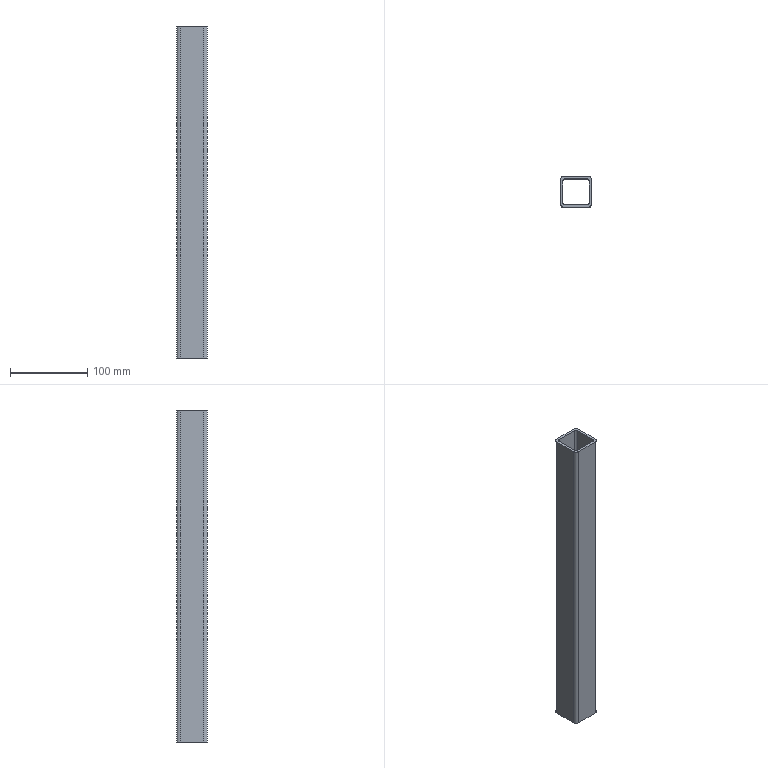Part | STEP file | DIN EN 10210-2 - 40 x 40 x 3 - 800 | 1 solid | 18 faces | box 40 x 40 x 429 mm | volume 186333 mm3 | plane 10 | cylinder 8 | commonest cylinder face diameters 6 x4 9 x4
STEP:
#1=CARTESIAN_POINT('',(0.,0.,0.));
#2=DIRECTION('',(0.,0.,1.));
#3=DIRECTION('',(1.,0.,0.));
#4=AXIS2_PLACEMENT_3D('',#1,#2,#3);
#5=CARTESIAN_POINT('',(17.,14.,0.));
#6=VERTEX_POINT('',#5);
#7=CARTESIAN_POINT('',(17.,14.,429.));
#8=VERTEX_POINT('',#7);
#9=CARTESIAN_POINT('',(17.,14.,0.));
#10=DIRECTION('',(0.,0.,1.));
#11=VECTOR('',#10,1.);
#12=LINE('',#9,#11);
#13=CARTESIAN_POINT('',(14.,14.,0.));
#14=DIRECTION('',(0.,0.,1.));
#15=DIRECTION('',(1.,0.,0.));
#16=AXIS2_PLACEMENT_3D('',#13,#14,#15);
#17=CYLINDRICAL_SURFACE('',#16,3.);
#18=CARTESIAN_POINT('',(0.,0.));
#19=DIRECTION('',(0.,1.));
#20=VECTOR('',#19,1.);
#21=LINE('',#18,#20);
#22=(GEOMETRIC_REPRESENTATION_CONTEXT(2)PARAMETRIC_REPRESENTATION_CONTEXT()REPRESENTATION_CONTEXT('',''));
#23=DEFINITIONAL_REPRESENTATION('',(#21),#22);
#24=PCURVE('',#17,#23);
#25=CARTESIAN_POINT('',(17.,14.,0.));
#26=DIRECTION('',(1.,0.,0.));
#27=DIRECTION('',(0.,0.,-1.));
#28=AXIS2_PLACEMENT_3D('',#25,#26,#27);
#29=PLANE('',#28);
#30=CARTESIAN_POINT('',(0.,0.));
#31=DIRECTION('',(-1.,0.));
#32=VECTOR('',#31,1.);
#33=LINE('',#30,#32);
#34=(GEOMETRIC_REPRESENTATION_CONTEXT(2)PARAMETRIC_REPRESENTATION_CONTEXT()REPRESENTATION_CONTEXT('',''));
#35=DEFINITIONAL_REPRESENTATION('',(#33),#34);
#36=PCURVE('',#29,#35);
#37=SURFACE_CURVE('',#12,(#24,#36),.PCURVE_S1.);
#38=EDGE_CURVE('',#6,#8,#37,.T.);
#39=ORIENTED_EDGE('',*,*,#38,.F.);
#40=CARTESIAN_POINT('',(14.,17.,0.));
#41=VERTEX_POINT('',#40);
#42=CARTESIAN_POINT('',(14.,14.,0.));
#43=DIRECTION('',(0.,0.,1.));
#44=DIRECTION('',(1.,0.,0.));
#45=AXIS2_PLACEMENT_3D('',#42,#43,#44);
#46=CIRCLE('',#45,3.);
#47=CARTESIAN_POINT('',(0.,0.));
#48=DIRECTION('',(1.,0.));
#49=VECTOR('',#48,1.);
#50=LINE('',#47,#49);
#51=(GEOMETRIC_REPRESENTATION_CONTEXT(2)PARAMETRIC_REPRESENTATION_CONTEXT()REPRESENTATION_CONTEXT('',''));
#52=DEFINITIONAL_REPRESENTATION('',(#50),#51);
#53=PCURVE('',#17,#52);
#54=CARTESIAN_POINT('',(0.,0.,0.));
#55=DIRECTION('',(0.,0.,1.));
#56=DIRECTION('',(1.,0.,0.));
#57=AXIS2_PLACEMENT_3D('',#54,#55,#56);
#58=PLANE('',#57);
#59=CARTESIAN_POINT('',(14.,14.));
#60=DIRECTION('',(1.,0.));
#61=AXIS2_PLACEMENT_2D('',#59,#60);
#62=CIRCLE('',#61,3.);
#63=(GEOMETRIC_REPRESENTATION_CONTEXT(2)PARAMETRIC_REPRESENTATION_CONTEXT()REPRESENTATION_CONTEXT('',''));
#64=DEFINITIONAL_REPRESENTATION('',(#62),#63);
#65=PCURVE('',#58,#64);
#66=SURFACE_CURVE('',#46,(#53,#65),.PCURVE_S1.);
#67=EDGE_CURVE('',#6,#41,#66,.T.);
#68=ORIENTED_EDGE('',*,*,#67,.T.);
#69=CARTESIAN_POINT('',(14.,17.,429.));
#70=VERTEX_POINT('',#69);
#71=CARTESIAN_POINT('',(14.,17.,0.));
#72=DIRECTION('',(0.,0.,1.));
#73=VECTOR('',#72,1.);
#74=LINE('',#71,#73);
#75=CARTESIAN_POINT('',(1.571,0.));
#76=DIRECTION('',(0.,1.));
#77=VECTOR('',#76,1.);
#78=LINE('',#75,#77);
#79=(GEOMETRIC_REPRESENTATION_CONTEXT(2)PARAMETRIC_REPRESENTATION_CONTEXT()REPRESENTATION_CONTEXT('',''));
#80=DEFINITIONAL_REPRESENTATION('',(#78),#79);
#81=PCURVE('',#17,#80);
#82=CARTESIAN_POINT('',(-14.,17.,0.));
#83=DIRECTION('',(0.,1.,0.));
#84=DIRECTION('',(0.,0.,1.));
#85=AXIS2_PLACEMENT_3D('',#82,#83,#84);
#86=PLANE('',#85);
#87=CARTESIAN_POINT('',(0.,28.));
#88=DIRECTION('',(1.,0.));
#89=VECTOR('',#88,1.);
#90=LINE('',#87,#89);
#91=(GEOMETRIC_REPRESENTATION_CONTEXT(2)PARAMETRIC_REPRESENTATION_CONTEXT()REPRESENTATION_CONTEXT('',''));
#92=DEFINITIONAL_REPRESENTATION('',(#90),#91);
#93=PCURVE('',#86,#92);
#94=SURFACE_CURVE('',#74,(#81,#93),.PCURVE_S1.);
#95=EDGE_CURVE('',#41,#70,#94,.T.);
#96=ORIENTED_EDGE('',*,*,#95,.T.);
#97=CARTESIAN_POINT('',(14.,14.,429.));
#98=DIRECTION('',(0.,0.,1.));
#99=DIRECTION('',(1.,0.,0.));
#100=AXIS2_PLACEMENT_3D('',#97,#98,#99);
#101=CIRCLE('',#100,3.);
#102=CARTESIAN_POINT('',(0.,429.));
#103=DIRECTION('',(1.,0.));
#104=VECTOR('',#103,1.);
#105=LINE('',#102,#104);
#106=(GEOMETRIC_REPRESENTATION_CONTEXT(2)PARAMETRIC_REPRESENTATION_CONTEXT()REPRESENTATION_CONTEXT('',''));
#107=DEFINITIONAL_REPRESENTATION('',(#105),#106);
#108=PCURVE('',#17,#107);
#109=CARTESIAN_POINT('',(0.,0.,429.));
#110=DIRECTION('',(0.,0.,1.));
#111=DIRECTION('',(1.,0.,0.));
#112=AXIS2_PLACEMENT_3D('',#109,#110,#111);
#113=PLANE('',#112);
#114=CARTESIAN_POINT('',(14.,14.));
#115=DIRECTION('',(1.,0.));
#116=AXIS2_PLACEMENT_2D('',#114,#115);
#117=CIRCLE('',#116,3.);
#118=(GEOMETRIC_REPRESENTATION_CONTEXT(2)PARAMETRIC_REPRESENTATION_CONTEXT()REPRESENTATION_CONTEXT('',''));
#119=DEFINITIONAL_REPRESENTATION('',(#117),#118);
#120=PCURVE('',#113,#119);
#121=SURFACE_CURVE('',#101,(#108,#120),.PCURVE_S1.);
#122=EDGE_CURVE('',#8,#70,#121,.T.);
#123=ORIENTED_EDGE('',*,*,#122,.F.);
#124=EDGE_LOOP('',(#39,#68,#96,#123));
#125=FACE_BOUND('',#124,.F.);
#126=ADVANCED_FACE('',(#125),#17,.F.);
#127=CARTESIAN_POINT('',(-14.,17.,429.));
#128=VERTEX_POINT('',#127);
#129=CARTESIAN_POINT('',(-7.,17.,429.));
#130=DIRECTION('',(-1.,0.,0.));
#131=VECTOR('',#130,1.);
#132=LINE('',#129,#131);
#133=CARTESIAN_POINT('',(429.,7.));
#134=DIRECTION('',(0.,-1.));
#135=VECTOR('',#134,1.);
#136=LINE('',#133,#135);
#137=(GEOMETRIC_REPRESENTATION_CONTEXT(2)PARAMETRIC_REPRESENTATION_CONTEXT()REPRESENTATION_CONTEXT('',''));
#138=DEFINITIONAL_REPRESENTATION('',(#136),#137);
#139=PCURVE('',#86,#138);
#140=CARTESIAN_POINT('',(-7.,17.));
#141=DIRECTION('',(-1.,0.));
#142=VECTOR('',#141,1.);
#143=LINE('',#140,#142);
#144=(GEOMETRIC_REPRESENTATION_CONTEXT(2)PARAMETRIC_REPRESENTATION_CONTEXT()REPRESENTATION_CONTEXT('',''));
#145=DEFINITIONAL_REPRESENTATION('',(#143),#144);
#146=PCURVE('',#113,#145);
#147=SURFACE_CURVE('',#132,(#139,#146),.PCURVE_S1.);
#148=EDGE_CURVE('',#70,#128,#147,.T.);
#149=ORIENTED_EDGE('',*,*,#148,.T.);
#150=CARTESIAN_POINT('',(-14.,17.,0.));
#151=VERTEX_POINT('',#150);
#152=CARTESIAN_POINT('',(-14.,17.,0.));
#153=DIRECTION('',(0.,0.,1.));
#154=VECTOR('',#153,1.);
#155=LINE('',#152,#154);
#156=CARTESIAN_POINT('',(0.,0.));
#157=DIRECTION('',(1.,0.));
#158=VECTOR('',#157,1.);
#159=LINE('',#156,#158);
#160=(GEOMETRIC_REPRESENTATION_CONTEXT(2)PARAMETRIC_REPRESENTATION_CONTEXT()REPRESENTATION_CONTEXT('',''));
#161=DEFINITIONAL_REPRESENTATION('',(#159),#160);
#162=PCURVE('',#86,#161);
#163=CARTESIAN_POINT('',(-14.,14.,0.));
#164=DIRECTION('',(0.,0.,1.));
#165=DIRECTION('',(0.,1.,0.));
#166=AXIS2_PLACEMENT_3D('',#163,#164,#165);
#167=CYLINDRICAL_SURFACE('',#166,3.);
#168=CARTESIAN_POINT('',(0.,0.));
#169=DIRECTION('',(0.,1.));
#170=VECTOR('',#169,1.);
#171=LINE('',#168,#170);
#172=(GEOMETRIC_REPRESENTATION_CONTEXT(2)PARAMETRIC_REPRESENTATION_CONTEXT()REPRESENTATION_CONTEXT('',''));
#173=DEFINITIONAL_REPRESENTATION('',(#171),#172);
#174=PCURVE('',#167,#173);
#175=SURFACE_CURVE('',#155,(#162,#174),.PCURVE_S1.);
#176=EDGE_CURVE('',#151,#128,#175,.T.);
#177=ORIENTED_EDGE('',*,*,#176,.F.);
#178=CARTESIAN_POINT('',(-7.,17.,0.));
#179=DIRECTION('',(-1.,0.,0.));
#180=VECTOR('',#179,1.);
#181=LINE('',#178,#180);
#182=CARTESIAN_POINT('',(0.,7.));
#183=DIRECTION('',(0.,-1.));
#184=VECTOR('',#183,1.);
#185=LINE('',#182,#184);
#186=(GEOMETRIC_REPRESENTATION_CONTEXT(2)PARAMETRIC_REPRESENTATION_CONTEXT()REPRESENTATION_CONTEXT('',''));
#187=DEFINITIONAL_REPRESENTATION('',(#185),#186);
#188=PCURVE('',#86,#187);
#189=CARTESIAN_POINT('',(-7.,17.));
#190=DIRECTION('',(-1.,0.));
#191=VECTOR('',#190,1.);
#192=LINE('',#189,#191);
#193=(GEOMETRIC_REPRESENTATION_CONTEXT(2)PARAMETRIC_REPRESENTATION_CONTEXT()REPRESENTATION_CONTEXT('',''));
#194=DEFINITIONAL_REPRESENTATION('',(#192),#193);
#195=PCURVE('',#58,#194);
#196=SURFACE_CURVE('',#181,(#188,#195),.PCURVE_S1.);
#197=EDGE_CURVE('',#41,#151,#196,.T.);
#198=ORIENTED_EDGE('',*,*,#197,.F.);
#199=ORIENTED_EDGE('',*,*,#95,.T.);
#200=EDGE_LOOP('',(#149,#177,#198,#199));
#201=FACE_BOUND('',#200,.T.);
#202=ADVANCED_FACE('',(#201),#86,.F.);
#203=ORIENTED_EDGE('',*,*,#176,.F.);
#204=CARTESIAN_POINT('',(-17.,14.,0.));
#205=VERTEX_POINT('',#204);
#206=CARTESIAN_POINT('',(-14.,14.,0.));
#207=DIRECTION('',(0.,0.,1.));
#208=DIRECTION('',(0.,1.,0.));
#209=AXIS2_PLACEMENT_3D('',#206,#207,#208);
#210=CIRCLE('',#209,3.);
#211=CARTESIAN_POINT('',(0.,0.));
#212=DIRECTION('',(1.,0.));
#213=VECTOR('',#212,1.);
#214=LINE('',#211,#213);
#215=(GEOMETRIC_REPRESENTATION_CONTEXT(2)PARAMETRIC_REPRESENTATION_CONTEXT()REPRESENTATION_CONTEXT('',''));
#216=DEFINITIONAL_REPRESENTATION('',(#214),#215);
#217=PCURVE('',#167,#216);
#218=CARTESIAN_POINT('',(-14.,14.));
#219=DIRECTION('',(0.,1.));
#220=AXIS2_PLACEMENT_2D('',#218,#219);
#221=CIRCLE('',#220,3.);
#222=(GEOMETRIC_REPRESENTATION_CONTEXT(2)PARAMETRIC_REPRESENTATION_CONTEXT()REPRESENTATION_CONTEXT('',''));
#223=DEFINITIONAL_REPRESENTATION('',(#221),#222);
#224=PCURVE('',#58,#223);
#225=SURFACE_CURVE('',#210,(#217,#224),.PCURVE_S1.);
#226=EDGE_CURVE('',#151,#205,#225,.T.);
#227=ORIENTED_EDGE('',*,*,#226,.T.);
#228=CARTESIAN_POINT('',(-17.,14.,429.));
#229=VERTEX_POINT('',#228);
#230=CARTESIAN_POINT('',(-17.,14.,0.));
#231=DIRECTION('',(0.,0.,1.));
#232=VECTOR('',#231,1.);
#233=LINE('',#230,#232);
#234=CARTESIAN_POINT('',(1.571,0.));
#235=DIRECTION('',(0.,1.));
#236=VECTOR('',#235,1.);
#237=LINE('',#234,#236);
#238=(GEOMETRIC_REPRESENTATION_CONTEXT(2)PARAMETRIC_REPRESENTATION_CONTEXT()REPRESENTATION_CONTEXT('',''));
#239=DEFINITIONAL_REPRESENTATION('',(#237),#238);
#240=PCURVE('',#167,#239);
#241=CARTESIAN_POINT('',(-17.,-14.,0.));
#242=DIRECTION('',(-1.,0.,0.));
#243=DIRECTION('',(0.,0.,1.));
#244=AXIS2_PLACEMENT_3D('',#241,#242,#243);
#245=PLANE('',#244);
#246=CARTESIAN_POINT('',(0.,28.));
#247=DIRECTION('',(1.,0.));
#248=VECTOR('',#247,1.);
#249=LINE('',#246,#248);
#250=(GEOMETRIC_REPRESENTATION_CONTEXT(2)PARAMETRIC_REPRESENTATION_CONTEXT()REPRESENTATION_CONTEXT('',''));
#251=DEFINITIONAL_REPRESENTATION('',(#249),#250);
#252=PCURVE('',#245,#251);
#253=SURFACE_CURVE('',#233,(#240,#252),.PCURVE_S1.);
#254=EDGE_CURVE('',#205,#229,#253,.T.);
#255=ORIENTED_EDGE('',*,*,#254,.T.);
#256=CARTESIAN_POINT('',(-14.,14.,429.));
#257=DIRECTION('',(0.,0.,1.));
#258=DIRECTION('',(0.,1.,0.));
#259=AXIS2_PLACEMENT_3D('',#256,#257,#258);
#260=CIRCLE('',#259,3.);
#261=CARTESIAN_POINT('',(0.,429.));
#262=DIRECTION('',(1.,0.));
#263=VECTOR('',#262,1.);
#264=LINE('',#261,#263);
#265=(GEOMETRIC_REPRESENTATION_CONTEXT(2)PARAMETRIC_REPRESENTATION_CONTEXT()REPRESENTATION_CONTEXT('',''));
#266=DEFINITIONAL_REPRESENTATION('',(#264),#265);
#267=PCURVE('',#167,#266);
#268=CARTESIAN_POINT('',(-14.,14.));
#269=DIRECTION('',(0.,1.));
#270=AXIS2_PLACEMENT_2D('',#268,#269);
#271=CIRCLE('',#270,3.);
#272=(GEOMETRIC_REPRESENTATION_CONTEXT(2)PARAMETRIC_REPRESENTATION_CONTEXT()REPRESENTATION_CONTEXT('',''));
#273=DEFINITIONAL_REPRESENTATION('',(#271),#272);
#274=PCURVE('',#113,#273);
#275=SURFACE_CURVE('',#260,(#267,#274),.PCURVE_S1.);
#276=EDGE_CURVE('',#128,#229,#275,.T.);
#277=ORIENTED_EDGE('',*,*,#276,.F.);
#278=EDGE_LOOP('',(#203,#227,#255,#277));
#279=FACE_BOUND('',#278,.F.);
#280=ADVANCED_FACE('',(#279),#167,.F.);
#281=CARTESIAN_POINT('',(-17.,-14.,429.));
#282=VERTEX_POINT('',#281);
#283=CARTESIAN_POINT('',(-17.,-7.,429.));
#284=DIRECTION('',(0.,-1.,0.));
#285=VECTOR('',#284,1.);
#286=LINE('',#283,#285);
#287=CARTESIAN_POINT('',(429.,7.));
#288=DIRECTION('',(0.,-1.));
#289=VECTOR('',#288,1.);
#290=LINE('',#287,#289);
#291=(GEOMETRIC_REPRESENTATION_CONTEXT(2)PARAMETRIC_REPRESENTATION_CONTEXT()REPRESENTATION_CONTEXT('',''));
#292=DEFINITIONAL_REPRESENTATION('',(#290),#291);
#293=PCURVE('',#245,#292);
#294=CARTESIAN_POINT('',(-17.,-7.));
#295=DIRECTION('',(0.,-1.));
#296=VECTOR('',#295,1.);
#297=LINE('',#294,#296);
#298=(GEOMETRIC_REPRESENTATION_CONTEXT(2)PARAMETRIC_REPRESENTATION_CONTEXT()REPRESENTATION_CONTEXT('',''));
#299=DEFINITIONAL_REPRESENTATION('',(#297),#298);
#300=PCURVE('',#113,#299);
#301=SURFACE_CURVE('',#286,(#293,#300),.PCURVE_S1.);
#302=EDGE_CURVE('',#229,#282,#301,.T.);
#303=ORIENTED_EDGE('',*,*,#302,.T.);
#304=CARTESIAN_POINT('',(-17.,-14.,0.));
#305=VERTEX_POINT('',#304);
#306=CARTESIAN_POINT('',(-17.,-14.,0.));
#307=DIRECTION('',(0.,0.,1.));
#308=VECTOR('',#307,1.);
#309=LINE('',#306,#308);
#310=CARTESIAN_POINT('',(0.,0.));
#311=DIRECTION('',(1.,0.));
#312=VECTOR('',#311,1.);
#313=LINE('',#310,#312);
#314=(GEOMETRIC_REPRESENTATION_CONTEXT(2)PARAMETRIC_REPRESENTATION_CONTEXT()REPRESENTATION_CONTEXT('',''));
#315=DEFINITIONAL_REPRESENTATION('',(#313),#314);
#316=PCURVE('',#245,#315);
#317=CARTESIAN_POINT('',(-14.,-14.,0.));
#318=DIRECTION('',(0.,0.,1.));
#319=DIRECTION('',(-1.,0.,0.));
#320=AXIS2_PLACEMENT_3D('',#317,#318,#319);
#321=CYLINDRICAL_SURFACE('',#320,3.);
#322=CARTESIAN_POINT('',(0.,0.));
#323=DIRECTION('',(0.,1.));
#324=VECTOR('',#323,1.);
#325=LINE('',#322,#324);
#326=(GEOMETRIC_REPRESENTATION_CONTEXT(2)PARAMETRIC_REPRESENTATION_CONTEXT()REPRESENTATION_CONTEXT('',''));
#327=DEFINITIONAL_REPRESENTATION('',(#325),#326);
#328=PCURVE('',#321,#327);
#329=SURFACE_CURVE('',#309,(#316,#328),.PCURVE_S1.);
#330=EDGE_CURVE('',#305,#282,#329,.T.);
#331=ORIENTED_EDGE('',*,*,#330,.F.);
#332=CARTESIAN_POINT('',(-17.,-7.,0.));
#333=DIRECTION('',(0.,-1.,0.));
#334=VECTOR('',#333,1.);
#335=LINE('',#332,#334);
#336=CARTESIAN_POINT('',(0.,7.));
#337=DIRECTION('',(0.,-1.));
#338=VECTOR('',#337,1.);
#339=LINE('',#336,#338);
#340=(GEOMETRIC_REPRESENTATION_CONTEXT(2)PARAMETRIC_REPRESENTATION_CONTEXT()REPRESENTATION_CONTEXT('',''));
#341=DEFINITIONAL_REPRESENTATION('',(#339),#340);
#342=PCURVE('',#245,#341);
#343=CARTESIAN_POINT('',(-17.,-7.));
#344=DIRECTION('',(0.,-1.));
#345=VECTOR('',#344,1.);
#346=LINE('',#343,#345);
#347=(GEOMETRIC_REPRESENTATION_CONTEXT(2)PARAMETRIC_REPRESENTATION_CONTEXT()REPRESENTATION_CONTEXT('',''));
#348=DEFINITIONAL_REPRESENTATION('',(#346),#347);
#349=PCURVE('',#58,#348);
#350=SURFACE_CURVE('',#335,(#342,#349),.PCURVE_S1.);
#351=EDGE_CURVE('',#205,#305,#350,.T.);
#352=ORIENTED_EDGE('',*,*,#351,.F.);
#353=ORIENTED_EDGE('',*,*,#254,.T.);
#354=EDGE_LOOP('',(#303,#331,#352,#353));
#355=FACE_BOUND('',#354,.T.);
#356=ADVANCED_FACE('',(#355),#245,.F.);
#357=CARTESIAN_POINT('',(20.,15.5,429.));
#358=VERTEX_POINT('',#357);
#359=CARTESIAN_POINT('',(20.,-15.5,429.));
#360=VERTEX_POINT('',#359);
#361=CARTESIAN_POINT('',(20.,7.75,429.));
#362=DIRECTION('',(0.,-1.,0.));
#363=VECTOR('',#362,1.);
#364=LINE('',#361,#363);
#365=CARTESIAN_POINT('',(20.,15.5,0.));
#366=DIRECTION('',(1.,0.,0.));
#367=DIRECTION('',(0.,0.,-1.));
#368=AXIS2_PLACEMENT_3D('',#365,#366,#367);
#369=PLANE('',#368);
#370=CARTESIAN_POINT('',(-429.,-7.75));
#371=DIRECTION('',(0.,-1.));
#372=VECTOR('',#371,1.);
#373=LINE('',#370,#372);
#374=(GEOMETRIC_REPRESENTATION_CONTEXT(2)PARAMETRIC_REPRESENTATION_CONTEXT()REPRESENTATION_CONTEXT('',''));
#375=DEFINITIONAL_REPRESENTATION('',(#373),#374);
#376=PCURVE('',#369,#375);
#377=CARTESIAN_POINT('',(20.,7.75));
#378=DIRECTION('',(0.,-1.));
#379=VECTOR('',#378,1.);
#380=LINE('',#377,#379);
#381=(GEOMETRIC_REPRESENTATION_CONTEXT(2)PARAMETRIC_REPRESENTATION_CONTEXT()REPRESENTATION_CONTEXT('',''));
#382=DEFINITIONAL_REPRESENTATION('',(#380),#381);
#383=PCURVE('',#113,#382);
#384=SURFACE_CURVE('',#364,(#376,#383),.PCURVE_S1.);
#385=EDGE_CURVE('',#358,#360,#384,.T.);
#386=ORIENTED_EDGE('',*,*,#385,.T.);
#387=CARTESIAN_POINT('',(20.,-15.5,0.));
#388=VERTEX_POINT('',#387);
#389=CARTESIAN_POINT('',(20.,-15.5,0.));
#390=DIRECTION('',(0.,0.,1.));
#391=VECTOR('',#390,1.);
#392=LINE('',#389,#391);
#393=CARTESIAN_POINT('',(0.,-31.));
#394=DIRECTION('',(-1.,0.));
#395=VECTOR('',#394,1.);
#396=LINE('',#393,#395);
#397=(GEOMETRIC_REPRESENTATION_CONTEXT(2)PARAMETRIC_REPRESENTATION_CONTEXT()REPRESENTATION_CONTEXT('',''));
#398=DEFINITIONAL_REPRESENTATION('',(#396),#397);
#399=PCURVE('',#369,#398);
#400=CARTESIAN_POINT('',(15.5,-15.5,0.));
#401=DIRECTION('',(0.,0.,1.));
#402=DIRECTION('',(0.,1.,0.));
#403=AXIS2_PLACEMENT_3D('',#400,#401,#402);
#404=CYLINDRICAL_SURFACE('',#403,4.5);
#405=CARTESIAN_POINT('',(4.712,0.));
#406=DIRECTION('',(0.,1.));
#407=VECTOR('',#406,1.);
#408=LINE('',#405,#407);
#409=(GEOMETRIC_REPRESENTATION_CONTEXT(2)PARAMETRIC_REPRESENTATION_CONTEXT()REPRESENTATION_CONTEXT('',''));
#410=DEFINITIONAL_REPRESENTATION('',(#408),#409);
#411=PCURVE('',#404,#410);
#412=SURFACE_CURVE('',#392,(#399,#411),.PCURVE_S1.);
#413=EDGE_CURVE('',#388,#360,#412,.T.);
#414=ORIENTED_EDGE('',*,*,#413,.F.);
#415=CARTESIAN_POINT('',(20.,15.5,0.));
#416=VERTEX_POINT('',#415);
#417=CARTESIAN_POINT('',(20.,7.75,0.));
#418=DIRECTION('',(0.,-1.,0.));
#419=VECTOR('',#418,1.);
#420=LINE('',#417,#419);
#421=CARTESIAN_POINT('',(0.,-7.75));
#422=DIRECTION('',(0.,-1.));
#423=VECTOR('',#422,1.);
#424=LINE('',#421,#423);
#425=(GEOMETRIC_REPRESENTATION_CONTEXT(2)PARAMETRIC_REPRESENTATION_CONTEXT()REPRESENTATION_CONTEXT('',''));
#426=DEFINITIONAL_REPRESENTATION('',(#424),#425);
#427=PCURVE('',#369,#426);
#428=CARTESIAN_POINT('',(20.,7.75));
#429=DIRECTION('',(0.,-1.));
#430=VECTOR('',#429,1.);
#431=LINE('',#428,#430);
#432=(GEOMETRIC_REPRESENTATION_CONTEXT(2)PARAMETRIC_REPRESENTATION_CONTEXT()REPRESENTATION_CONTEXT('',''));
#433=DEFINITIONAL_REPRESENTATION('',(#431),#432);
#434=PCURVE('',#58,#433);
#435=SURFACE_CURVE('',#420,(#427,#434),.PCURVE_S1.);
#436=EDGE_CURVE('',#416,#388,#435,.T.);
#437=ORIENTED_EDGE('',*,*,#436,.F.);
#438=CARTESIAN_POINT('',(20.,15.5,0.));
#439=DIRECTION('',(0.,0.,1.));
#440=VECTOR('',#439,1.);
#441=LINE('',#438,#440);
#442=CARTESIAN_POINT('',(0.,0.));
#443=DIRECTION('',(-1.,0.));
#444=VECTOR('',#443,1.);
#445=LINE('',#442,#444);
#446=(GEOMETRIC_REPRESENTATION_CONTEXT(2)PARAMETRIC_REPRESENTATION_CONTEXT()REPRESENTATION_CONTEXT('',''));
#447=DEFINITIONAL_REPRESENTATION('',(#445),#446);
#448=PCURVE('',#369,#447);
#449=CARTESIAN_POINT('',(15.5,15.5,0.));
#450=DIRECTION('',(0.,0.,1.));
#451=DIRECTION('',(-1.,0.,0.));
#452=AXIS2_PLACEMENT_3D('',#449,#450,#451);
#453=CYLINDRICAL_SURFACE('',#452,4.5);
#454=CARTESIAN_POINT('',(3.142,0.));
#455=DIRECTION('',(0.,1.));
#456=VECTOR('',#455,1.);
#457=LINE('',#454,#456);
#458=(GEOMETRIC_REPRESENTATION_CONTEXT(2)PARAMETRIC_REPRESENTATION_CONTEXT()REPRESENTATION_CONTEXT('',''));
#459=DEFINITIONAL_REPRESENTATION('',(#457),#458);
#460=PCURVE('',#453,#459);
#461=SURFACE_CURVE('',#441,(#448,#460),.PCURVE_S1.);
#462=EDGE_CURVE('',#416,#358,#461,.T.);
#463=ORIENTED_EDGE('',*,*,#462,.T.);
#464=EDGE_LOOP('',(#386,#414,#437,#463));
#465=FACE_BOUND('',#464,.T.);
#466=ADVANCED_FACE('',(#465),#369,.T.);
#467=CARTESIAN_POINT('',(15.5,-20.,429.));
#468=VERTEX_POINT('',#467);
#469=CARTESIAN_POINT('',(15.5,-15.5,429.));
#470=DIRECTION('',(0.,0.,-1.));
#471=DIRECTION('',(0.,1.,0.));
#472=AXIS2_PLACEMENT_3D('',#469,#470,#471);
#473=CIRCLE('',#472,4.5);
#474=CARTESIAN_POINT('',(6.283,429.));
#475=DIRECTION('',(-1.,0.));
#476=VECTOR('',#475,1.);
#477=LINE('',#474,#476);
#478=(GEOMETRIC_REPRESENTATION_CONTEXT(2)PARAMETRIC_REPRESENTATION_CONTEXT()REPRESENTATION_CONTEXT('',''));
#479=DEFINITIONAL_REPRESENTATION('',(#477),#478);
#480=PCURVE('',#404,#479);
#481=CARTESIAN_POINT('',(15.5,-11.));
#482=CARTESIAN_POINT('',(23.294,-11.));
#483=CARTESIAN_POINT('',(19.397,-17.75));
#484=CARTESIAN_POINT('',(15.5,-24.5));
#485=CARTESIAN_POINT('',(11.603,-17.75));
#486=CARTESIAN_POINT('',(7.706,-11.));
#487=CARTESIAN_POINT('',(15.5,-11.));
#488=(BOUNDED_CURVE()B_SPLINE_CURVE(2,(#481,#482,#483,#484,#485,#486,#487),.UNSPECIFIED.,.T.,.F.)B_SPLINE_CURVE_WITH_KNOTS((1,2,2,2,2,1),(-2.094,0.,2.094,4.189,6.283,8.378),.UNSPECIFIED.)CURVE()GEOMETRIC_REPRESENTATION_ITEM()RATIONAL_B_SPLINE_CURVE((1.,0.5,1.,0.5,1.,0.5,1.))REPRESENTATION_ITEM(''));
#489=(GEOMETRIC_REPRESENTATION_CONTEXT(2)PARAMETRIC_REPRESENTATION_CONTEXT()REPRESENTATION_CONTEXT('',''));
#490=DEFINITIONAL_REPRESENTATION('',(#488),#489);
#491=PCURVE('',#113,#490);
#492=SURFACE_CURVE('',#473,(#480,#491),.PCURVE_S1.);
#493=EDGE_CURVE('',#360,#468,#492,.T.);
#494=ORIENTED_EDGE('',*,*,#493,.T.);
#495=CARTESIAN_POINT('',(15.5,-20.,0.));
#496=VERTEX_POINT('',#495);
#497=CARTESIAN_POINT('',(15.5,-20.,0.));
#498=DIRECTION('',(0.,0.,1.));
#499=VECTOR('',#498,1.);
#500=LINE('',#497,#499);
#501=CARTESIAN_POINT('',(3.142,0.));
#502=DIRECTION('',(0.,1.));
#503=VECTOR('',#502,1.);
#504=LINE('',#501,#503);
#505=(GEOMETRIC_REPRESENTATION_CONTEXT(2)PARAMETRIC_REPRESENTATION_CONTEXT()REPRESENTATION_CONTEXT('',''));
#506=DEFINITIONAL_REPRESENTATION('',(#504),#505);
#507=PCURVE('',#404,#506);
#508=CARTESIAN_POINT('',(15.5,-20.,0.));
#509=DIRECTION('',(0.,-1.,0.));
#510=DIRECTION('',(0.,0.,-1.));
#511=AXIS2_PLACEMENT_3D('',#508,#509,#510);
#512=PLANE('',#511);
#513=CARTESIAN_POINT('',(0.,0.));
#514=DIRECTION('',(-1.,0.));
#515=VECTOR('',#514,1.);
#516=LINE('',#513,#515);
#517=(GEOMETRIC_REPRESENTATION_CONTEXT(2)PARAMETRIC_REPRESENTATION_CONTEXT()REPRESENTATION_CONTEXT('',''));
#518=DEFINITIONAL_REPRESENTATION('',(#516),#517);
#519=PCURVE('',#512,#518);
#520=SURFACE_CURVE('',#500,(#507,#519),.PCURVE_S1.);
#521=EDGE_CURVE('',#496,#468,#520,.T.);
#522=ORIENTED_EDGE('',*,*,#521,.F.);
#523=CARTESIAN_POINT('',(15.5,-15.5,0.));
#524=DIRECTION('',(0.,0.,-1.));
#525=DIRECTION('',(0.,1.,0.));
#526=AXIS2_PLACEMENT_3D('',#523,#524,#525);
#527=CIRCLE('',#526,4.5);
#528=CARTESIAN_POINT('',(6.283,0.));
#529=DIRECTION('',(-1.,0.));
#530=VECTOR('',#529,1.);
#531=LINE('',#528,#530);
#532=(GEOMETRIC_REPRESENTATION_CONTEXT(2)PARAMETRIC_REPRESENTATION_CONTEXT()REPRESENTATION_CONTEXT('',''));
#533=DEFINITIONAL_REPRESENTATION('',(#531),#532);
#534=PCURVE('',#404,#533);
#535=CARTESIAN_POINT('',(15.5,-11.));
#536=CARTESIAN_POINT('',(23.294,-11.));
#537=CARTESIAN_POINT('',(19.397,-17.75));
#538=CARTESIAN_POINT('',(15.5,-24.5));
#539=CARTESIAN_POINT('',(11.603,-17.75));
#540=CARTESIAN_POINT('',(7.706,-11.));
#541=CARTESIAN_POINT('',(15.5,-11.));
#542=(BOUNDED_CURVE()B_SPLINE_CURVE(2,(#535,#536,#537,#538,#539,#540,#541),.UNSPECIFIED.,.T.,.F.)B_SPLINE_CURVE_WITH_KNOTS((1,2,2,2,2,1),(-2.094,0.,2.094,4.189,6.283,8.378),.UNSPECIFIED.)CURVE()GEOMETRIC_REPRESENTATION_ITEM()RATIONAL_B_SPLINE_CURVE((1.,0.5,1.,0.5,1.,0.5,1.))REPRESENTATION_ITEM(''));
#543=(GEOMETRIC_REPRESENTATION_CONTEXT(2)PARAMETRIC_REPRESENTATION_CONTEXT()REPRESENTATION_CONTEXT('',''));
#544=DEFINITIONAL_REPRESENTATION('',(#542),#543);
#545=PCURVE('',#58,#544);
#546=SURFACE_CURVE('',#527,(#534,#545),.PCURVE_S1.);
#547=EDGE_CURVE('',#388,#496,#546,.T.);
#548=ORIENTED_EDGE('',*,*,#547,.F.);
#549=ORIENTED_EDGE('',*,*,#413,.T.);
#550=EDGE_LOOP('',(#494,#522,#548,#549));
#551=FACE_BOUND('',#550,.T.);
#552=ADVANCED_FACE('',(#551),#404,.T.);
#553=CARTESIAN_POINT('',(-15.5,-20.,429.));
#554=VERTEX_POINT('',#553);
#555=CARTESIAN_POINT('',(7.75,-20.,429.));
#556=DIRECTION('',(-1.,0.,0.));
#557=VECTOR('',#556,1.);
#558=LINE('',#555,#557);
#559=CARTESIAN_POINT('',(-429.,-7.75));
#560=DIRECTION('',(0.,-1.));
#561=VECTOR('',#560,1.);
#562=LINE('',#559,#561);
#563=(GEOMETRIC_REPRESENTATION_CONTEXT(2)PARAMETRIC_REPRESENTATION_CONTEXT()REPRESENTATION_CONTEXT('',''));
#564=DEFINITIONAL_REPRESENTATION('',(#562),#563);
#565=PCURVE('',#512,#564);
#566=CARTESIAN_POINT('',(7.75,-20.));
#567=DIRECTION('',(-1.,0.));
#568=VECTOR('',#567,1.);
#569=LINE('',#566,#568);
#570=(GEOMETRIC_REPRESENTATION_CONTEXT(2)PARAMETRIC_REPRESENTATION_CONTEXT()REPRESENTATION_CONTEXT('',''));
#571=DEFINITIONAL_REPRESENTATION('',(#569),#570);
#572=PCURVE('',#113,#571);
#573=SURFACE_CURVE('',#558,(#565,#572),.PCURVE_S1.);
#574=EDGE_CURVE('',#468,#554,#573,.T.);
#575=ORIENTED_EDGE('',*,*,#574,.T.);
#576=CARTESIAN_POINT('',(-15.5,-20.,0.));
#577=VERTEX_POINT('',#576);
#578=CARTESIAN_POINT('',(-15.5,-20.,0.));
#579=DIRECTION('',(0.,0.,1.));
#580=VECTOR('',#579,1.);
#581=LINE('',#578,#580);
#582=CARTESIAN_POINT('',(0.,-31.));
#583=DIRECTION('',(-1.,0.));
#584=VECTOR('',#583,1.);
#585=LINE('',#582,#584);
#586=(GEOMETRIC_REPRESENTATION_CONTEXT(2)PARAMETRIC_REPRESENTATION_CONTEXT()REPRESENTATION_CONTEXT('',''));
#587=DEFINITIONAL_REPRESENTATION('',(#585),#586);
#588=PCURVE('',#512,#587);
#589=CARTESIAN_POINT('',(-15.5,-15.5,0.));
#590=DIRECTION('',(0.,0.,1.));
#591=DIRECTION('',(1.,0.,0.));
#592=AXIS2_PLACEMENT_3D('',#589,#590,#591);
#593=CYLINDRICAL_SURFACE('',#592,4.5);
#594=CARTESIAN_POINT('',(4.712,0.));
#595=DIRECTION('',(0.,1.));
#596=VECTOR('',#595,1.);
#597=LINE('',#594,#596);
#598=(GEOMETRIC_REPRESENTATION_CONTEXT(2)PARAMETRIC_REPRESENTATION_CONTEXT()REPRESENTATION_CONTEXT('',''));
#599=DEFINITIONAL_REPRESENTATION('',(#597),#598);
#600=PCURVE('',#593,#599);
#601=SURFACE_CURVE('',#581,(#588,#600),.PCURVE_S1.);
#602=EDGE_CURVE('',#577,#554,#601,.T.);
#603=ORIENTED_EDGE('',*,*,#602,.F.);
#604=CARTESIAN_POINT('',(7.75,-20.,0.));
#605=DIRECTION('',(-1.,0.,0.));
#606=VECTOR('',#605,1.);
#607=LINE('',#604,#606);
#608=CARTESIAN_POINT('',(0.,-7.75));
#609=DIRECTION('',(0.,-1.));
#610=VECTOR('',#609,1.);
#611=LINE('',#608,#610);
#612=(GEOMETRIC_REPRESENTATION_CONTEXT(2)PARAMETRIC_REPRESENTATION_CONTEXT()REPRESENTATION_CONTEXT('',''));
#613=DEFINITIONAL_REPRESENTATION('',(#611),#612);
#614=PCURVE('',#512,#613);
#615=CARTESIAN_POINT('',(7.75,-20.));
#616=DIRECTION('',(-1.,0.));
#617=VECTOR('',#616,1.);
#618=LINE('',#615,#617);
#619=(GEOMETRIC_REPRESENTATION_CONTEXT(2)PARAMETRIC_REPRESENTATION_CONTEXT()REPRESENTATION_CONTEXT('',''));
#620=DEFINITIONAL_REPRESENTATION('',(#618),#619);
#621=PCURVE('',#58,#620);
#622=SURFACE_CURVE('',#607,(#614,#621),.PCURVE_S1.);
#623=EDGE_CURVE('',#496,#577,#622,.T.);
#624=ORIENTED_EDGE('',*,*,#623,.F.);
#625=ORIENTED_EDGE('',*,*,#521,.T.);
#626=EDGE_LOOP('',(#575,#603,#624,#625));
#627=FACE_BOUND('',#626,.T.);
#628=ADVANCED_FACE('',(#627),#512,.T.);
#629=CARTESIAN_POINT('',(-20.,-15.5,429.));
#630=VERTEX_POINT('',#629);
#631=CARTESIAN_POINT('',(-15.5,-15.5,429.));
#632=DIRECTION('',(0.,0.,-1.));
#633=DIRECTION('',(1.,0.,0.));
#634=AXIS2_PLACEMENT_3D('',#631,#632,#633);
#635=CIRCLE('',#634,4.5);
#636=CARTESIAN_POINT('',(6.283,429.));
#637=DIRECTION('',(-1.,0.));
#638=VECTOR('',#637,1.);
#639=LINE('',#636,#638);
#640=(GEOMETRIC_REPRESENTATION_CONTEXT(2)PARAMETRIC_REPRESENTATION_CONTEXT()REPRESENTATION_CONTEXT('',''));
#641=DEFINITIONAL_REPRESENTATION('',(#639),#640);
#642=PCURVE('',#593,#641);
#643=CARTESIAN_POINT('',(-11.,-15.5));
#644=CARTESIAN_POINT('',(-11.,-23.294));
#645=CARTESIAN_POINT('',(-17.75,-19.397));
#646=CARTESIAN_POINT('',(-24.5,-15.5));
#647=CARTESIAN_POINT('',(-17.75,-11.603));
#648=CARTESIAN_POINT('',(-11.,-7.706));
#649=CARTESIAN_POINT('',(-11.,-15.5));
#650=(BOUNDED_CURVE()B_SPLINE_CURVE(2,(#643,#644,#645,#646,#647,#648,#649),.UNSPECIFIED.,.T.,.F.)B_SPLINE_CURVE_WITH_KNOTS((1,2,2,2,2,1),(-2.094,0.,2.094,4.189,6.283,8.378),.UNSPECIFIED.)CURVE()GEOMETRIC_REPRESENTATION_ITEM()RATIONAL_B_SPLINE_CURVE((1.,0.5,1.,0.5,1.,0.5,1.))REPRESENTATION_ITEM(''));
#651=(GEOMETRIC_REPRESENTATION_CONTEXT(2)PARAMETRIC_REPRESENTATION_CONTEXT()REPRESENTATION_CONTEXT('',''));
#652=DEFINITIONAL_REPRESENTATION('',(#650),#651);
#653=PCURVE('',#113,#652);
#654=SURFACE_CURVE('',#635,(#642,#653),.PCURVE_S1.);
#655=EDGE_CURVE('',#554,#630,#654,.T.);
#656=ORIENTED_EDGE('',*,*,#655,.T.);
#657=CARTESIAN_POINT('',(-20.,-15.5,0.));
#658=VERTEX_POINT('',#657);
#659=CARTESIAN_POINT('',(-20.,-15.5,0.));
#660=DIRECTION('',(0.,0.,1.));
#661=VECTOR('',#660,1.);
#662=LINE('',#659,#661);
#663=CARTESIAN_POINT('',(3.142,0.));
#664=DIRECTION('',(0.,1.));
#665=VECTOR('',#664,1.);
#666=LINE('',#663,#665);
#667=(GEOMETRIC_REPRESENTATION_CONTEXT(2)PARAMETRIC_REPRESENTATION_CONTEXT()REPRESENTATION_CONTEXT('',''));
#668=DEFINITIONAL_REPRESENTATION('',(#666),#667);
#669=PCURVE('',#593,#668);
#670=CARTESIAN_POINT('',(-20.,-15.5,0.));
#671=DIRECTION('',(-1.,0.,0.));
#672=DIRECTION('',(0.,0.,1.));
#673=AXIS2_PLACEMENT_3D('',#670,#671,#672);
#674=PLANE('',#673);
#675=CARTESIAN_POINT('',(0.,0.));
#676=DIRECTION('',(1.,0.));
#677=VECTOR('',#676,1.);
#678=LINE('',#675,#677);
#679=(GEOMETRIC_REPRESENTATION_CONTEXT(2)PARAMETRIC_REPRESENTATION_CONTEXT()REPRESENTATION_CONTEXT('',''));
#680=DEFINITIONAL_REPRESENTATION('',(#678),#679);
#681=PCURVE('',#674,#680);
#682=SURFACE_CURVE('',#662,(#669,#681),.PCURVE_S1.);
#683=EDGE_CURVE('',#658,#630,#682,.T.);
#684=ORIENTED_EDGE('',*,*,#683,.F.);
#685=CARTESIAN_POINT('',(-15.5,-15.5,0.));
#686=DIRECTION('',(0.,0.,-1.));
#687=DIRECTION('',(1.,0.,0.));
#688=AXIS2_PLACEMENT_3D('',#685,#686,#687);
#689=CIRCLE('',#688,4.5);
#690=CARTESIAN_POINT('',(6.283,0.));
#691=DIRECTION('',(-1.,0.));
#692=VECTOR('',#691,1.);
#693=LINE('',#690,#692);
#694=(GEOMETRIC_REPRESENTATION_CONTEXT(2)PARAMETRIC_REPRESENTATION_CONTEXT()REPRESENTATION_CONTEXT('',''));
#695=DEFINITIONAL_REPRESENTATION('',(#693),#694);
#696=PCURVE('',#593,#695);
#697=CARTESIAN_POINT('',(-11.,-15.5));
#698=CARTESIAN_POINT('',(-11.,-23.294));
#699=CARTESIAN_POINT('',(-17.75,-19.397));
#700=CARTESIAN_POINT('',(-24.5,-15.5));
#701=CARTESIAN_POINT('',(-17.75,-11.603));
#702=CARTESIAN_POINT('',(-11.,-7.706));
#703=CARTESIAN_POINT('',(-11.,-15.5));
#704=(BOUNDED_CURVE()B_SPLINE_CURVE(2,(#697,#698,#699,#700,#701,#702,#703),.UNSPECIFIED.,.T.,.F.)B_SPLINE_CURVE_WITH_KNOTS((1,2,2,2,2,1),(-2.094,0.,2.094,4.189,6.283,8.378),.UNSPECIFIED.)CURVE()GEOMETRIC_REPRESENTATION_ITEM()RATIONAL_B_SPLINE_CURVE((1.,0.5,1.,0.5,1.,0.5,1.))REPRESENTATION_ITEM(''));
#705=(GEOMETRIC_REPRESENTATION_CONTEXT(2)PARAMETRIC_REPRESENTATION_CONTEXT()REPRESENTATION_CONTEXT('',''));
#706=DEFINITIONAL_REPRESENTATION('',(#704),#705);
#707=PCURVE('',#58,#706);
#708=SURFACE_CURVE('',#689,(#696,#707),.PCURVE_S1.);
#709=EDGE_CURVE('',#577,#658,#708,.T.);
#710=ORIENTED_EDGE('',*,*,#709,.F.);
#711=ORIENTED_EDGE('',*,*,#602,.T.);
#712=EDGE_LOOP('',(#656,#684,#710,#711));
#713=FACE_BOUND('',#712,.T.);
#714=ADVANCED_FACE('',(#713),#593,.T.);
#715=ORIENTED_EDGE('',*,*,#330,.F.);
#716=CARTESIAN_POINT('',(-14.,-17.,0.));
#717=VERTEX_POINT('',#716);
#718=CARTESIAN_POINT('',(-14.,-14.,0.));
#719=DIRECTION('',(0.,0.,1.));
#720=DIRECTION('',(-1.,0.,0.));
#721=AXIS2_PLACEMENT_3D('',#718,#719,#720);
#722=CIRCLE('',#721,3.);
#723=CARTESIAN_POINT('',(0.,0.));
#724=DIRECTION('',(1.,0.));
#725=VECTOR('',#724,1.);
#726=LINE('',#723,#725);
#727=(GEOMETRIC_REPRESENTATION_CONTEXT(2)PARAMETRIC_REPRESENTATION_CONTEXT()REPRESENTATION_CONTEXT('',''));
#728=DEFINITIONAL_REPRESENTATION('',(#726),#727);
#729=PCURVE('',#321,#728);
#730=CARTESIAN_POINT('',(-14.,-14.));
#731=DIRECTION('',(-1.,0.));
#732=AXIS2_PLACEMENT_2D('',#730,#731);
#733=CIRCLE('',#732,3.);
#734=(GEOMETRIC_REPRESENTATION_CONTEXT(2)PARAMETRIC_REPRESENTATION_CONTEXT()REPRESENTATION_CONTEXT('',''));
#735=DEFINITIONAL_REPRESENTATION('',(#733),#734);
#736=PCURVE('',#58,#735);
#737=SURFACE_CURVE('',#722,(#729,#736),.PCURVE_S1.);
#738=EDGE_CURVE('',#305,#717,#737,.T.);
#739=ORIENTED_EDGE('',*,*,#738,.T.);
#740=CARTESIAN_POINT('',(-14.,-17.,429.));
#741=VERTEX_POINT('',#740);
#742=CARTESIAN_POINT('',(-14.,-17.,0.));
#743=DIRECTION('',(0.,0.,1.));
#744=VECTOR('',#743,1.);
#745=LINE('',#742,#744);
#746=CARTESIAN_POINT('',(1.571,0.));
#747=DIRECTION('',(0.,1.));
#748=VECTOR('',#747,1.);
#749=LINE('',#746,#748);
#750=(GEOMETRIC_REPRESENTATION_CONTEXT(2)PARAMETRIC_REPRESENTATION_CONTEXT()REPRESENTATION_CONTEXT('',''));
#751=DEFINITIONAL_REPRESENTATION('',(#749),#750);
#752=PCURVE('',#321,#751);
#753=CARTESIAN_POINT('',(14.,-17.,0.));
#754=DIRECTION('',(0.,-1.,0.));
#755=DIRECTION('',(0.,0.,-1.));
#756=AXIS2_PLACEMENT_3D('',#753,#754,#755);
#757=PLANE('',#756);
#758=CARTESIAN_POINT('',(0.,-28.));
#759=DIRECTION('',(-1.,0.));
#760=VECTOR('',#759,1.);
#761=LINE('',#758,#760);
#762=(GEOMETRIC_REPRESENTATION_CONTEXT(2)PARAMETRIC_REPRESENTATION_CONTEXT()REPRESENTATION_CONTEXT('',''));
#763=DEFINITIONAL_REPRESENTATION('',(#761),#762);
#764=PCURVE('',#757,#763);
#765=SURFACE_CURVE('',#745,(#752,#764),.PCURVE_S1.);
#766=EDGE_CURVE('',#717,#741,#765,.T.);
#767=ORIENTED_EDGE('',*,*,#766,.T.);
#768=CARTESIAN_POINT('',(-14.,-14.,429.));
#769=DIRECTION('',(0.,0.,1.));
#770=DIRECTION('',(-1.,0.,0.));
#771=AXIS2_PLACEMENT_3D('',#768,#769,#770);
#772=CIRCLE('',#771,3.);
#773=CARTESIAN_POINT('',(0.,429.));
#774=DIRECTION('',(1.,0.));
#775=VECTOR('',#774,1.);
#776=LINE('',#773,#775);
#777=(GEOMETRIC_REPRESENTATION_CONTEXT(2)PARAMETRIC_REPRESENTATION_CONTEXT()REPRESENTATION_CONTEXT('',''));
#778=DEFINITIONAL_REPRESENTATION('',(#776),#777);
#779=PCURVE('',#321,#778);
#780=CARTESIAN_POINT('',(-14.,-14.));
#781=DIRECTION('',(-1.,0.));
#782=AXIS2_PLACEMENT_2D('',#780,#781);
#783=CIRCLE('',#782,3.);
#784=(GEOMETRIC_REPRESENTATION_CONTEXT(2)PARAMETRIC_REPRESENTATION_CONTEXT()REPRESENTATION_CONTEXT('',''));
#785=DEFINITIONAL_REPRESENTATION('',(#783),#784);
#786=PCURVE('',#113,#785);
#787=SURFACE_CURVE('',#772,(#779,#786),.PCURVE_S1.);
#788=EDGE_CURVE('',#282,#741,#787,.T.);
#789=ORIENTED_EDGE('',*,*,#788,.F.);
#790=EDGE_LOOP('',(#715,#739,#767,#789));
#791=FACE_BOUND('',#790,.F.);
#792=ADVANCED_FACE('',(#791),#321,.F.);
#793=CARTESIAN_POINT('',(17.,-14.,429.));
#794=VERTEX_POINT('',#793);
#795=CARTESIAN_POINT('',(17.,7.,429.));
#796=DIRECTION('',(0.,1.,0.));
#797=VECTOR('',#796,1.);
#798=LINE('',#795,#797);
#799=CARTESIAN_POINT('',(-429.,-7.));
#800=DIRECTION('',(0.,1.));
#801=VECTOR('',#800,1.);
#802=LINE('',#799,#801);
#803=(GEOMETRIC_REPRESENTATION_CONTEXT(2)PARAMETRIC_REPRESENTATION_CONTEXT()REPRESENTATION_CONTEXT('',''));
#804=DEFINITIONAL_REPRESENTATION('',(#802),#803);
#805=PCURVE('',#29,#804);
#806=CARTESIAN_POINT('',(17.,7.));
#807=DIRECTION('',(0.,1.));
#808=VECTOR('',#807,1.);
#809=LINE('',#806,#808);
#810=(GEOMETRIC_REPRESENTATION_CONTEXT(2)PARAMETRIC_REPRESENTATION_CONTEXT()REPRESENTATION_CONTEXT('',''));
#811=DEFINITIONAL_REPRESENTATION('',(#809),#810);
#812=PCURVE('',#113,#811);
#813=SURFACE_CURVE('',#798,(#805,#812),.PCURVE_S1.);
#814=EDGE_CURVE('',#794,#8,#813,.T.);
#815=ORIENTED_EDGE('',*,*,#814,.T.);
#816=ORIENTED_EDGE('',*,*,#38,.F.);
#817=CARTESIAN_POINT('',(17.,-14.,0.));
#818=VERTEX_POINT('',#817);
#819=CARTESIAN_POINT('',(17.,7.,0.));
#820=DIRECTION('',(0.,1.,0.));
#821=VECTOR('',#820,1.);
#822=LINE('',#819,#821);
#823=CARTESIAN_POINT('',(0.,-7.));
#824=DIRECTION('',(0.,1.));
#825=VECTOR('',#824,1.);
#826=LINE('',#823,#825);
#827=(GEOMETRIC_REPRESENTATION_CONTEXT(2)PARAMETRIC_REPRESENTATION_CONTEXT()REPRESENTATION_CONTEXT('',''));
#828=DEFINITIONAL_REPRESENTATION('',(#826),#827);
#829=PCURVE('',#29,#828);
#830=CARTESIAN_POINT('',(17.,7.));
#831=DIRECTION('',(0.,1.));
#832=VECTOR('',#831,1.);
#833=LINE('',#830,#832);
#834=(GEOMETRIC_REPRESENTATION_CONTEXT(2)PARAMETRIC_REPRESENTATION_CONTEXT()REPRESENTATION_CONTEXT('',''));
#835=DEFINITIONAL_REPRESENTATION('',(#833),#834);
#836=PCURVE('',#58,#835);
#837=SURFACE_CURVE('',#822,(#829,#836),.PCURVE_S1.);
#838=EDGE_CURVE('',#818,#6,#837,.T.);
#839=ORIENTED_EDGE('',*,*,#838,.F.);
#840=CARTESIAN_POINT('',(17.,-14.,0.));
#841=DIRECTION('',(0.,0.,1.));
#842=VECTOR('',#841,1.);
#843=LINE('',#840,#842);
#844=CARTESIAN_POINT('',(0.,-28.));
#845=DIRECTION('',(-1.,0.));
#846=VECTOR('',#845,1.);
#847=LINE('',#844,#846);
#848=(GEOMETRIC_REPRESENTATION_CONTEXT(2)PARAMETRIC_REPRESENTATION_CONTEXT()REPRESENTATION_CONTEXT('',''));
#849=DEFINITIONAL_REPRESENTATION('',(#847),#848);
#850=PCURVE('',#29,#849);
#851=CARTESIAN_POINT('',(14.,-14.,0.));
#852=DIRECTION('',(0.,0.,1.));
#853=DIRECTION('',(0.,-1.,0.));
#854=AXIS2_PLACEMENT_3D('',#851,#852,#853);
#855=CYLINDRICAL_SURFACE('',#854,3.);
#856=CARTESIAN_POINT('',(1.571,0.));
#857=DIRECTION('',(0.,1.));
#858=VECTOR('',#857,1.);
#859=LINE('',#856,#858);
#860=(GEOMETRIC_REPRESENTATION_CONTEXT(2)PARAMETRIC_REPRESENTATION_CONTEXT()REPRESENTATION_CONTEXT('',''));
#861=DEFINITIONAL_REPRESENTATION('',(#859),#860);
#862=PCURVE('',#855,#861);
#863=SURFACE_CURVE('',#843,(#850,#862),.PCURVE_S1.);
#864=EDGE_CURVE('',#818,#794,#863,.T.);
#865=ORIENTED_EDGE('',*,*,#864,.T.);
#866=EDGE_LOOP('',(#815,#816,#839,#865));
#867=FACE_BOUND('',#866,.T.);
#868=ADVANCED_FACE('',(#867),#29,.F.);
#869=CARTESIAN_POINT('',(14.,-17.,0.));
#870=VERTEX_POINT('',#869);
#871=CARTESIAN_POINT('',(14.,-17.,429.));
#872=VERTEX_POINT('',#871);
#873=CARTESIAN_POINT('',(14.,-17.,0.));
#874=DIRECTION('',(0.,0.,1.));
#875=VECTOR('',#874,1.);
#876=LINE('',#873,#875);
#877=CARTESIAN_POINT('',(0.,0.));
#878=DIRECTION('',(0.,1.));
#879=VECTOR('',#878,1.);
#880=LINE('',#877,#879);
#881=(GEOMETRIC_REPRESENTATION_CONTEXT(2)PARAMETRIC_REPRESENTATION_CONTEXT()REPRESENTATION_CONTEXT('',''));
#882=DEFINITIONAL_REPRESENTATION('',(#880),#881);
#883=PCURVE('',#855,#882);
#884=CARTESIAN_POINT('',(0.,0.));
#885=DIRECTION('',(-1.,0.));
#886=VECTOR('',#885,1.);
#887=LINE('',#884,#886);
#888=(GEOMETRIC_REPRESENTATION_CONTEXT(2)PARAMETRIC_REPRESENTATION_CONTEXT()REPRESENTATION_CONTEXT('',''));
#889=DEFINITIONAL_REPRESENTATION('',(#887),#888);
#890=PCURVE('',#757,#889);
#891=SURFACE_CURVE('',#876,(#883,#890),.PCURVE_S1.);
#892=EDGE_CURVE('',#870,#872,#891,.T.);
#893=ORIENTED_EDGE('',*,*,#892,.F.);
#894=CARTESIAN_POINT('',(14.,-14.,0.));
#895=DIRECTION('',(0.,0.,1.));
#896=DIRECTION('',(0.,-1.,0.));
#897=AXIS2_PLACEMENT_3D('',#894,#895,#896);
#898=CIRCLE('',#897,3.);
#899=CARTESIAN_POINT('',(0.,0.));
#900=DIRECTION('',(1.,0.));
#901=VECTOR('',#900,1.);
#902=LINE('',#899,#901);
#903=(GEOMETRIC_REPRESENTATION_CONTEXT(2)PARAMETRIC_REPRESENTATION_CONTEXT()REPRESENTATION_CONTEXT('',''));
#904=DEFINITIONAL_REPRESENTATION('',(#902),#903);
#905=PCURVE('',#855,#904);
#906=CARTESIAN_POINT('',(14.,-14.));
#907=DIRECTION('',(0.,-1.));
#908=AXIS2_PLACEMENT_2D('',#906,#907);
#909=CIRCLE('',#908,3.);
#910=(GEOMETRIC_REPRESENTATION_CONTEXT(2)PARAMETRIC_REPRESENTATION_CONTEXT()REPRESENTATION_CONTEXT('',''));
#911=DEFINITIONAL_REPRESENTATION('',(#909),#910);
#912=PCURVE('',#58,#911);
#913=SURFACE_CURVE('',#898,(#905,#912),.PCURVE_S1.);
#914=EDGE_CURVE('',#870,#818,#913,.T.);
#915=ORIENTED_EDGE('',*,*,#914,.T.);
#916=ORIENTED_EDGE('',*,*,#864,.T.);
#917=CARTESIAN_POINT('',(14.,-14.,429.));
#918=DIRECTION('',(0.,0.,1.));
#919=DIRECTION('',(0.,-1.,0.));
#920=AXIS2_PLACEMENT_3D('',#917,#918,#919);
#921=CIRCLE('',#920,3.);
#922=CARTESIAN_POINT('',(0.,429.));
#923=DIRECTION('',(1.,0.));
#924=VECTOR('',#923,1.);
#925=LINE('',#922,#924);
#926=(GEOMETRIC_REPRESENTATION_CONTEXT(2)PARAMETRIC_REPRESENTATION_CONTEXT()REPRESENTATION_CONTEXT('',''));
#927=DEFINITIONAL_REPRESENTATION('',(#925),#926);
#928=PCURVE('',#855,#927);
#929=CARTESIAN_POINT('',(14.,-14.));
#930=DIRECTION('',(0.,-1.));
#931=AXIS2_PLACEMENT_2D('',#929,#930);
#932=CIRCLE('',#931,3.);
#933=(GEOMETRIC_REPRESENTATION_CONTEXT(2)PARAMETRIC_REPRESENTATION_CONTEXT()REPRESENTATION_CONTEXT('',''));
#934=DEFINITIONAL_REPRESENTATION('',(#932),#933);
#935=PCURVE('',#113,#934);
#936=SURFACE_CURVE('',#921,(#928,#935),.PCURVE_S1.);
#937=EDGE_CURVE('',#872,#794,#936,.T.);
#938=ORIENTED_EDGE('',*,*,#937,.F.);
#939=EDGE_LOOP('',(#893,#915,#916,#938));
#940=FACE_BOUND('',#939,.F.);
#941=ADVANCED_FACE('',(#940),#855,.F.);
#942=CARTESIAN_POINT('',(7.,-17.,429.));
#943=DIRECTION('',(1.,0.,0.));
#944=VECTOR('',#943,1.);
#945=LINE('',#942,#944);
#946=CARTESIAN_POINT('',(-429.,-7.));
#947=DIRECTION('',(0.,1.));
#948=VECTOR('',#947,1.);
#949=LINE('',#946,#948);
#950=(GEOMETRIC_REPRESENTATION_CONTEXT(2)PARAMETRIC_REPRESENTATION_CONTEXT()REPRESENTATION_CONTEXT('',''));
#951=DEFINITIONAL_REPRESENTATION('',(#949),#950);
#952=PCURVE('',#757,#951);
#953=CARTESIAN_POINT('',(7.,-17.));
#954=DIRECTION('',(1.,0.));
#955=VECTOR('',#954,1.);
#956=LINE('',#953,#955);
#957=(GEOMETRIC_REPRESENTATION_CONTEXT(2)PARAMETRIC_REPRESENTATION_CONTEXT()REPRESENTATION_CONTEXT('',''));
#958=DEFINITIONAL_REPRESENTATION('',(#956),#957);
#959=PCURVE('',#113,#958);
#960=SURFACE_CURVE('',#945,(#952,#959),.PCURVE_S1.);
#961=EDGE_CURVE('',#741,#872,#960,.T.);
#962=ORIENTED_EDGE('',*,*,#961,.T.);
#963=ORIENTED_EDGE('',*,*,#892,.F.);
#964=CARTESIAN_POINT('',(7.,-17.,0.));
#965=DIRECTION('',(1.,0.,0.));
#966=VECTOR('',#965,1.);
#967=LINE('',#964,#966);
#968=CARTESIAN_POINT('',(0.,-7.));
#969=DIRECTION('',(0.,1.));
#970=VECTOR('',#969,1.);
#971=LINE('',#968,#970);
#972=(GEOMETRIC_REPRESENTATION_CONTEXT(2)PARAMETRIC_REPRESENTATION_CONTEXT()REPRESENTATION_CONTEXT('',''));
#973=DEFINITIONAL_REPRESENTATION('',(#971),#972);
#974=PCURVE('',#757,#973);
#975=CARTESIAN_POINT('',(7.,-17.));
#976=DIRECTION('',(1.,0.));
#977=VECTOR('',#976,1.);
#978=LINE('',#975,#977);
#979=(GEOMETRIC_REPRESENTATION_CONTEXT(2)PARAMETRIC_REPRESENTATION_CONTEXT()REPRESENTATION_CONTEXT('',''));
#980=DEFINITIONAL_REPRESENTATION('',(#978),#979);
#981=PCURVE('',#58,#980);
#982=SURFACE_CURVE('',#967,(#974,#981),.PCURVE_S1.);
#983=EDGE_CURVE('',#717,#870,#982,.T.);
#984=ORIENTED_EDGE('',*,*,#983,.F.);
#985=ORIENTED_EDGE('',*,*,#766,.T.);
#986=EDGE_LOOP('',(#962,#963,#984,#985));
#987=FACE_BOUND('',#986,.T.);
#988=ADVANCED_FACE('',(#987),#757,.F.);
#989=CARTESIAN_POINT('',(-20.,15.5,429.));
#990=VERTEX_POINT('',#989);
#991=CARTESIAN_POINT('',(-20.,-7.75,429.));
#992=DIRECTION('',(0.,1.,0.));
#993=VECTOR('',#992,1.);
#994=LINE('',#991,#993);
#995=CARTESIAN_POINT('',(429.,7.75));
#996=DIRECTION('',(0.,1.));
#997=VECTOR('',#996,1.);
#998=LINE('',#995,#997);
#999=(GEOMETRIC_REPRESENTATION_CONTEXT(2)PARAMETRIC_REPRESENTATION_CONTEXT()REPRESENTATION_CONTEXT('',''));
#1000=DEFINITIONAL_REPRESENTATION('',(#998),#999);
#1001=PCURVE('',#674,#1000);
#1002=CARTESIAN_POINT('',(-20.,-7.75));
#1003=DIRECTION('',(0.,1.));
#1004=VECTOR('',#1003,1.);
#1005=LINE('',#1002,#1004);
#1006=(GEOMETRIC_REPRESENTATION_CONTEXT(2)PARAMETRIC_REPRESENTATION_CONTEXT()REPRESENTATION_CONTEXT('',''));
#1007=DEFINITIONAL_REPRESENTATION('',(#1005),#1006);
#1008=PCURVE('',#113,#1007);
#1009=SURFACE_CURVE('',#994,(#1001,#1008),.PCURVE_S1.);
#1010=EDGE_CURVE('',#630,#990,#1009,.T.);
#1011=ORIENTED_EDGE('',*,*,#1010,.T.);
#1012=CARTESIAN_POINT('',(-20.,15.5,0.));
#1013=VERTEX_POINT('',#1012);
#1014=CARTESIAN_POINT('',(-20.,15.5,0.));
#1015=DIRECTION('',(0.,0.,1.));
#1016=VECTOR('',#1015,1.);
#1017=LINE('',#1014,#1016);
#1018=CARTESIAN_POINT('',(0.,31.));
#1019=DIRECTION('',(1.,0.));
#1020=VECTOR('',#1019,1.);
#1021=LINE('',#1018,#1020);
#1022=(GEOMETRIC_REPRESENTATION_CONTEXT(2)PARAMETRIC_REPRESENTATION_CONTEXT()REPRESENTATION_CONTEXT('',''));
#1023=DEFINITIONAL_REPRESENTATION('',(#1021),#1022);
#1024=PCURVE('',#674,#1023);
#1025=CARTESIAN_POINT('',(-15.5,15.5,0.));
#1026=DIRECTION('',(0.,0.,1.));
#1027=DIRECTION('',(0.,-1.,0.));
#1028=AXIS2_PLACEMENT_3D('',#1025,#1026,#1027);
#1029=CYLINDRICAL_SURFACE('',#1028,4.5);
#1030=CARTESIAN_POINT('',(4.712,0.));
#1031=DIRECTION('',(0.,1.));
#1032=VECTOR('',#1031,1.);
#1033=LINE('',#1030,#1032);
#1034=(GEOMETRIC_REPRESENTATION_CONTEXT(2)PARAMETRIC_REPRESENTATION_CONTEXT()REPRESENTATION_CONTEXT('',''));
#1035=DEFINITIONAL_REPRESENTATION('',(#1033),#1034);
#1036=PCURVE('',#1029,#1035);
#1037=SURFACE_CURVE('',#1017,(#1024,#1036),.PCURVE_S1.);
#1038=EDGE_CURVE('',#1013,#990,#1037,.T.);
#1039=ORIENTED_EDGE('',*,*,#1038,.F.);
#1040=CARTESIAN_POINT('',(-20.,-7.75,0.));
#1041=DIRECTION('',(0.,1.,0.));
#1042=VECTOR('',#1041,1.);
#1043=LINE('',#1040,#1042);
#1044=CARTESIAN_POINT('',(0.,7.75));
#1045=DIRECTION('',(0.,1.));
#1046=VECTOR('',#1045,1.);
#1047=LINE('',#1044,#1046);
#1048=(GEOMETRIC_REPRESENTATION_CONTEXT(2)PARAMETRIC_REPRESENTATION_CONTEXT()REPRESENTATION_CONTEXT('',''));
#1049=DEFINITIONAL_REPRESENTATION('',(#1047),#1048);
#1050=PCURVE('',#674,#1049);
#1051=CARTESIAN_POINT('',(-20.,-7.75));
#1052=DIRECTION('',(0.,1.));
#1053=VECTOR('',#1052,1.);
#1054=LINE('',#1051,#1053);
#1055=(GEOMETRIC_REPRESENTATION_CONTEXT(2)PARAMETRIC_REPRESENTATION_CONTEXT()REPRESENTATION_CONTEXT('',''));
#1056=DEFINITIONAL_REPRESENTATION('',(#1054),#1055);
#1057=PCURVE('',#58,#1056);
#1058=SURFACE_CURVE('',#1043,(#1050,#1057),.PCURVE_S1.);
#1059=EDGE_CURVE('',#658,#1013,#1058,.T.);
#1060=ORIENTED_EDGE('',*,*,#1059,.F.);
#1061=ORIENTED_EDGE('',*,*,#683,.T.);
#1062=EDGE_LOOP('',(#1011,#1039,#1060,#1061));
#1063=FACE_BOUND('',#1062,.T.);
#1064=ADVANCED_FACE('',(#1063),#674,.T.);
#1065=CARTESIAN_POINT('',(-15.5,20.,429.));
#1066=VERTEX_POINT('',#1065);
#1067=CARTESIAN_POINT('',(-15.5,15.5,429.));
#1068=DIRECTION('',(0.,0.,-1.));
#1069=DIRECTION('',(0.,-1.,0.));
#1070=AXIS2_PLACEMENT_3D('',#1067,#1068,#1069);
#1071=CIRCLE('',#1070,4.5);
#1072=CARTESIAN_POINT('',(6.283,429.));
#1073=DIRECTION('',(-1.,0.));
#1074=VECTOR('',#1073,1.);
#1075=LINE('',#1072,#1074);
#1076=(GEOMETRIC_REPRESENTATION_CONTEXT(2)PARAMETRIC_REPRESENTATION_CONTEXT()REPRESENTATION_CONTEXT('',''));
#1077=DEFINITIONAL_REPRESENTATION('',(#1075),#1076);
#1078=PCURVE('',#1029,#1077);
#1079=CARTESIAN_POINT('',(-15.5,11.));
#1080=CARTESIAN_POINT('',(-23.294,11.));
#1081=CARTESIAN_POINT('',(-19.397,17.75));
#1082=CARTESIAN_POINT('',(-15.5,24.5));
#1083=CARTESIAN_POINT('',(-11.603,17.75));
#1084=CARTESIAN_POINT('',(-7.706,11.));
#1085=CARTESIAN_POINT('',(-15.5,11.));
#1086=(BOUNDED_CURVE()B_SPLINE_CURVE(2,(#1079,#1080,#1081,#1082,#1083,#1084,#1085),.UNSPECIFIED.,.T.,.F.)B_SPLINE_CURVE_WITH_KNOTS((1,2,2,2,2,1),(-2.094,0.,2.094,4.189,6.283,8.378),.UNSPECIFIED.)CURVE()GEOMETRIC_REPRESENTATION_ITEM()RATIONAL_B_SPLINE_CURVE((1.,0.5,1.,0.5,1.,0.5,1.))REPRESENTATION_ITEM(''));
#1087=(GEOMETRIC_REPRESENTATION_CONTEXT(2)PARAMETRIC_REPRESENTATION_CONTEXT()REPRESENTATION_CONTEXT('',''));
#1088=DEFINITIONAL_REPRESENTATION('',(#1086),#1087);
#1089=PCURVE('',#113,#1088);
#1090=SURFACE_CURVE('',#1071,(#1078,#1089),.PCURVE_S1.);
#1091=EDGE_CURVE('',#990,#1066,#1090,.T.);
#1092=ORIENTED_EDGE('',*,*,#1091,.T.);
#1093=CARTESIAN_POINT('',(-15.5,20.,0.));
#1094=VERTEX_POINT('',#1093);
#1095=CARTESIAN_POINT('',(-15.5,20.,0.));
#1096=DIRECTION('',(0.,0.,1.));
#1097=VECTOR('',#1096,1.);
#1098=LINE('',#1095,#1097);
#1099=CARTESIAN_POINT('',(3.142,0.));
#1100=DIRECTION('',(0.,1.));
#1101=VECTOR('',#1100,1.);
#1102=LINE('',#1099,#1101);
#1103=(GEOMETRIC_REPRESENTATION_CONTEXT(2)PARAMETRIC_REPRESENTATION_CONTEXT()REPRESENTATION_CONTEXT('',''));
#1104=DEFINITIONAL_REPRESENTATION('',(#1102),#1103);
#1105=PCURVE('',#1029,#1104);
#1106=CARTESIAN_POINT('',(-15.5,20.,0.));
#1107=DIRECTION('',(0.,1.,0.));
#1108=DIRECTION('',(0.,0.,1.));
#1109=AXIS2_PLACEMENT_3D('',#1106,#1107,#1108);
#1110=PLANE('',#1109);
#1111=CARTESIAN_POINT('',(0.,0.));
#1112=DIRECTION('',(1.,0.));
#1113=VECTOR('',#1112,1.);
#1114=LINE('',#1111,#1113);
#1115=(GEOMETRIC_REPRESENTATION_CONTEXT(2)PARAMETRIC_REPRESENTATION_CONTEXT()REPRESENTATION_CONTEXT('',''));
#1116=DEFINITIONAL_REPRESENTATION('',(#1114),#1115);
#1117=PCURVE('',#1110,#1116);
#1118=SURFACE_CURVE('',#1098,(#1105,#1117),.PCURVE_S1.);
#1119=EDGE_CURVE('',#1094,#1066,#1118,.T.);
#1120=ORIENTED_EDGE('',*,*,#1119,.F.);
#1121=CARTESIAN_POINT('',(-15.5,15.5,0.));
#1122=DIRECTION('',(0.,0.,-1.));
#1123=DIRECTION('',(0.,-1.,0.));
#1124=AXIS2_PLACEMENT_3D('',#1121,#1122,#1123);
#1125=CIRCLE('',#1124,4.5);
#1126=CARTESIAN_POINT('',(6.283,0.));
#1127=DIRECTION('',(-1.,0.));
#1128=VECTOR('',#1127,1.);
#1129=LINE('',#1126,#1128);
#1130=(GEOMETRIC_REPRESENTATION_CONTEXT(2)PARAMETRIC_REPRESENTATION_CONTEXT()REPRESENTATION_CONTEXT('',''));
#1131=DEFINITIONAL_REPRESENTATION('',(#1129),#1130);
#1132=PCURVE('',#1029,#1131);
#1133=CARTESIAN_POINT('',(-15.5,11.));
#1134=CARTESIAN_POINT('',(-23.294,11.));
#1135=CARTESIAN_POINT('',(-19.397,17.75));
#1136=CARTESIAN_POINT('',(-15.5,24.5));
#1137=CARTESIAN_POINT('',(-11.603,17.75));
#1138=CARTESIAN_POINT('',(-7.706,11.));
#1139=CARTESIAN_POINT('',(-15.5,11.));
#1140=(BOUNDED_CURVE()B_SPLINE_CURVE(2,(#1133,#1134,#1135,#1136,#1137,#1138,#1139),.UNSPECIFIED.,.T.,.F.)B_SPLINE_CURVE_WITH_KNOTS((1,2,2,2,2,1),(-2.094,0.,2.094,4.189,6.283,8.378),.UNSPECIFIED.)CURVE()GEOMETRIC_REPRESENTATION_ITEM()RATIONAL_B_SPLINE_CURVE((1.,0.5,1.,0.5,1.,0.5,1.))REPRESENTATION_ITEM(''));
#1141=(GEOMETRIC_REPRESENTATION_CONTEXT(2)PARAMETRIC_REPRESENTATION_CONTEXT()REPRESENTATION_CONTEXT('',''));
#1142=DEFINITIONAL_REPRESENTATION('',(#1140),#1141);
#1143=PCURVE('',#58,#1142);
#1144=SURFACE_CURVE('',#1125,(#1132,#1143),.PCURVE_S1.);
#1145=EDGE_CURVE('',#1013,#1094,#1144,.T.);
#1146=ORIENTED_EDGE('',*,*,#1145,.F.);
#1147=ORIENTED_EDGE('',*,*,#1038,.T.);
#1148=EDGE_LOOP('',(#1092,#1120,#1146,#1147));
#1149=FACE_BOUND('',#1148,.T.);
#1150=ADVANCED_FACE('',(#1149),#1029,.T.);
#1151=CARTESIAN_POINT('',(15.5,20.,429.));
#1152=VERTEX_POINT('',#1151);
#1153=CARTESIAN_POINT('',(-7.75,20.,429.));
#1154=DIRECTION('',(1.,0.,0.));
#1155=VECTOR('',#1154,1.);
#1156=LINE('',#1153,#1155);
#1157=CARTESIAN_POINT('',(429.,7.75));
#1158=DIRECTION('',(0.,1.));
#1159=VECTOR('',#1158,1.);
#1160=LINE('',#1157,#1159);
#1161=(GEOMETRIC_REPRESENTATION_CONTEXT(2)PARAMETRIC_REPRESENTATION_CONTEXT()REPRESENTATION_CONTEXT('',''));
#1162=DEFINITIONAL_REPRESENTATION('',(#1160),#1161);
#1163=PCURVE('',#1110,#1162);
#1164=CARTESIAN_POINT('',(-7.75,20.));
#1165=DIRECTION('',(1.,0.));
#1166=VECTOR('',#1165,1.);
#1167=LINE('',#1164,#1166);
#1168=(GEOMETRIC_REPRESENTATION_CONTEXT(2)PARAMETRIC_REPRESENTATION_CONTEXT()REPRESENTATION_CONTEXT('',''));
#1169=DEFINITIONAL_REPRESENTATION('',(#1167),#1168);
#1170=PCURVE('',#113,#1169);
#1171=SURFACE_CURVE('',#1156,(#1163,#1170),.PCURVE_S1.);
#1172=EDGE_CURVE('',#1066,#1152,#1171,.T.);
#1173=ORIENTED_EDGE('',*,*,#1172,.T.);
#1174=CARTESIAN_POINT('',(15.5,20.,0.));
#1175=VERTEX_POINT('',#1174);
#1176=CARTESIAN_POINT('',(15.5,20.,0.));
#1177=DIRECTION('',(0.,0.,1.));
#1178=VECTOR('',#1177,1.);
#1179=LINE('',#1176,#1178);
#1180=CARTESIAN_POINT('',(0.,31.));
#1181=DIRECTION('',(1.,0.));
#1182=VECTOR('',#1181,1.);
#1183=LINE('',#1180,#1182);
#1184=(GEOMETRIC_REPRESENTATION_CONTEXT(2)PARAMETRIC_REPRESENTATION_CONTEXT()REPRESENTATION_CONTEXT('',''));
#1185=DEFINITIONAL_REPRESENTATION('',(#1183),#1184);
#1186=PCURVE('',#1110,#1185);
#1187=CARTESIAN_POINT('',(4.712,0.));
#1188=DIRECTION('',(0.,1.));
#1189=VECTOR('',#1188,1.);
#1190=LINE('',#1187,#1189);
#1191=(GEOMETRIC_REPRESENTATION_CONTEXT(2)PARAMETRIC_REPRESENTATION_CONTEXT()REPRESENTATION_CONTEXT('',''));
#1192=DEFINITIONAL_REPRESENTATION('',(#1190),#1191);
#1193=PCURVE('',#453,#1192);
#1194=SURFACE_CURVE('',#1179,(#1186,#1193),.PCURVE_S1.);
#1195=EDGE_CURVE('',#1175,#1152,#1194,.T.);
#1196=ORIENTED_EDGE('',*,*,#1195,.F.);
#1197=CARTESIAN_POINT('',(-7.75,20.,0.));
#1198=DIRECTION('',(1.,0.,0.));
#1199=VECTOR('',#1198,1.);
#1200=LINE('',#1197,#1199);
#1201=CARTESIAN_POINT('',(0.,7.75));
#1202=DIRECTION('',(0.,1.));
#1203=VECTOR('',#1202,1.);
#1204=LINE('',#1201,#1203);
#1205=(GEOMETRIC_REPRESENTATION_CONTEXT(2)PARAMETRIC_REPRESENTATION_CONTEXT()REPRESENTATION_CONTEXT('',''));
#1206=DEFINITIONAL_REPRESENTATION('',(#1204),#1205);
#1207=PCURVE('',#1110,#1206);
#1208=CARTESIAN_POINT('',(-7.75,20.));
#1209=DIRECTION('',(1.,0.));
#1210=VECTOR('',#1209,1.);
#1211=LINE('',#1208,#1210);
#1212=(GEOMETRIC_REPRESENTATION_CONTEXT(2)PARAMETRIC_REPRESENTATION_CONTEXT()REPRESENTATION_CONTEXT('',''));
#1213=DEFINITIONAL_REPRESENTATION('',(#1211),#1212);
#1214=PCURVE('',#58,#1213);
#1215=SURFACE_CURVE('',#1200,(#1207,#1214),.PCURVE_S1.);
#1216=EDGE_CURVE('',#1094,#1175,#1215,.T.);
#1217=ORIENTED_EDGE('',*,*,#1216,.F.);
#1218=ORIENTED_EDGE('',*,*,#1119,.T.);
#1219=EDGE_LOOP('',(#1173,#1196,#1217,#1218));
#1220=FACE_BOUND('',#1219,.T.);
#1221=ADVANCED_FACE('',(#1220),#1110,.T.);
#1222=CARTESIAN_POINT('',(15.5,15.5,429.));
#1223=DIRECTION('',(0.,0.,-1.));
#1224=DIRECTION('',(-1.,0.,0.));
#1225=AXIS2_PLACEMENT_3D('',#1222,#1223,#1224);
#1226=CIRCLE('',#1225,4.5);
#1227=CARTESIAN_POINT('',(6.283,429.));
#1228=DIRECTION('',(-1.,0.));
#1229=VECTOR('',#1228,1.);
#1230=LINE('',#1227,#1229);
#1231=(GEOMETRIC_REPRESENTATION_CONTEXT(2)PARAMETRIC_REPRESENTATION_CONTEXT()REPRESENTATION_CONTEXT('',''));
#1232=DEFINITIONAL_REPRESENTATION('',(#1230),#1231);
#1233=PCURVE('',#453,#1232);
#1234=CARTESIAN_POINT('',(11.,15.5));
#1235=CARTESIAN_POINT('',(11.,23.294));
#1236=CARTESIAN_POINT('',(17.75,19.397));
#1237=CARTESIAN_POINT('',(24.5,15.5));
#1238=CARTESIAN_POINT('',(17.75,11.603));
#1239=CARTESIAN_POINT('',(11.,7.706));
#1240=CARTESIAN_POINT('',(11.,15.5));
#1241=(BOUNDED_CURVE()B_SPLINE_CURVE(2,(#1234,#1235,#1236,#1237,#1238,#1239,#1240),.UNSPECIFIED.,.T.,.F.)B_SPLINE_CURVE_WITH_KNOTS((1,2,2,2,2,1),(-2.094,0.,2.094,4.189,6.283,8.378),.UNSPECIFIED.)CURVE()GEOMETRIC_REPRESENTATION_ITEM()RATIONAL_B_SPLINE_CURVE((1.,0.5,1.,0.5,1.,0.5,1.))REPRESENTATION_ITEM(''));
#1242=(GEOMETRIC_REPRESENTATION_CONTEXT(2)PARAMETRIC_REPRESENTATION_CONTEXT()REPRESENTATION_CONTEXT('',''));
#1243=DEFINITIONAL_REPRESENTATION('',(#1241),#1242);
#1244=PCURVE('',#113,#1243);
#1245=SURFACE_CURVE('',#1226,(#1233,#1244),.PCURVE_S1.);
#1246=EDGE_CURVE('',#1152,#358,#1245,.T.);
#1247=ORIENTED_EDGE('',*,*,#1246,.T.);
#1248=ORIENTED_EDGE('',*,*,#462,.F.);
#1249=CARTESIAN_POINT('',(15.5,15.5,0.));
#1250=DIRECTION('',(0.,0.,-1.));
#1251=DIRECTION('',(-1.,0.,0.));
#1252=AXIS2_PLACEMENT_3D('',#1249,#1250,#1251);
#1253=CIRCLE('',#1252,4.5);
#1254=CARTESIAN_POINT('',(6.283,0.));
#1255=DIRECTION('',(-1.,0.));
#1256=VECTOR('',#1255,1.);
#1257=LINE('',#1254,#1256);
#1258=(GEOMETRIC_REPRESENTATION_CONTEXT(2)PARAMETRIC_REPRESENTATION_CONTEXT()REPRESENTATION_CONTEXT('',''));
#1259=DEFINITIONAL_REPRESENTATION('',(#1257),#1258);
#1260=PCURVE('',#453,#1259);
#1261=CARTESIAN_POINT('',(11.,15.5));
#1262=CARTESIAN_POINT('',(11.,23.294));
#1263=CARTESIAN_POINT('',(17.75,19.397));
#1264=CARTESIAN_POINT('',(24.5,15.5));
#1265=CARTESIAN_POINT('',(17.75,11.603));
#1266=CARTESIAN_POINT('',(11.,7.706));
#1267=CARTESIAN_POINT('',(11.,15.5));
#1268=(BOUNDED_CURVE()B_SPLINE_CURVE(2,(#1261,#1262,#1263,#1264,#1265,#1266,#1267),.UNSPECIFIED.,.T.,.F.)B_SPLINE_CURVE_WITH_KNOTS((1,2,2,2,2,1),(-2.094,0.,2.094,4.189,6.283,8.378),.UNSPECIFIED.)CURVE()GEOMETRIC_REPRESENTATION_ITEM()RATIONAL_B_SPLINE_CURVE((1.,0.5,1.,0.5,1.,0.5,1.))REPRESENTATION_ITEM(''));
#1269=(GEOMETRIC_REPRESENTATION_CONTEXT(2)PARAMETRIC_REPRESENTATION_CONTEXT()REPRESENTATION_CONTEXT('',''));
#1270=DEFINITIONAL_REPRESENTATION('',(#1268),#1269);
#1271=PCURVE('',#58,#1270);
#1272=SURFACE_CURVE('',#1253,(#1260,#1271),.PCURVE_S1.);
#1273=EDGE_CURVE('',#1175,#416,#1272,.T.);
#1274=ORIENTED_EDGE('',*,*,#1273,.F.);
#1275=ORIENTED_EDGE('',*,*,#1195,.T.);
#1276=EDGE_LOOP('',(#1247,#1248,#1274,#1275));
#1277=FACE_BOUND('',#1276,.T.);
#1278=ADVANCED_FACE('',(#1277),#453,.T.);
#1279=ORIENTED_EDGE('',*,*,#1059,.T.);
#1280=ORIENTED_EDGE('',*,*,#1145,.T.);
#1281=ORIENTED_EDGE('',*,*,#1216,.T.);
#1282=ORIENTED_EDGE('',*,*,#1273,.T.);
#1283=ORIENTED_EDGE('',*,*,#436,.T.);
#1284=ORIENTED_EDGE('',*,*,#547,.T.);
#1285=ORIENTED_EDGE('',*,*,#623,.T.);
#1286=ORIENTED_EDGE('',*,*,#709,.T.);
#1287=EDGE_LOOP('',(#1279,#1280,#1281,#1282,#1283,#1284,#1285,#1286));
#1288=FACE_BOUND('',#1287,.T.);
#1289=ORIENTED_EDGE('',*,*,#738,.T.);
#1290=ORIENTED_EDGE('',*,*,#983,.T.);
#1291=ORIENTED_EDGE('',*,*,#914,.T.);
#1292=ORIENTED_EDGE('',*,*,#838,.T.);
#1293=ORIENTED_EDGE('',*,*,#67,.T.);
#1294=ORIENTED_EDGE('',*,*,#197,.T.);
#1295=ORIENTED_EDGE('',*,*,#226,.T.);
#1296=ORIENTED_EDGE('',*,*,#351,.T.);
#1297=EDGE_LOOP('',(#1289,#1290,#1291,#1292,#1293,#1294,#1295,#1296));
#1298=FACE_BOUND('',#1297,.T.);
#1299=ADVANCED_FACE('',(#1288,#1298),#58,.F.);
#1300=ORIENTED_EDGE('',*,*,#1010,.F.);
#1301=ORIENTED_EDGE('',*,*,#655,.F.);
#1302=ORIENTED_EDGE('',*,*,#574,.F.);
#1303=ORIENTED_EDGE('',*,*,#493,.F.);
#1304=ORIENTED_EDGE('',*,*,#385,.F.);
#1305=ORIENTED_EDGE('',*,*,#1246,.F.);
#1306=ORIENTED_EDGE('',*,*,#1172,.F.);
#1307=ORIENTED_EDGE('',*,*,#1091,.F.);
#1308=EDGE_LOOP('',(#1300,#1301,#1302,#1303,#1304,#1305,#1306,#1307));
#1309=FACE_BOUND('',#1308,.T.);
#1310=ORIENTED_EDGE('',*,*,#788,.F.);
#1311=ORIENTED_EDGE('',*,*,#302,.F.);
#1312=ORIENTED_EDGE('',*,*,#276,.F.);
#1313=ORIENTED_EDGE('',*,*,#148,.F.);
#1314=ORIENTED_EDGE('',*,*,#122,.F.);
#1315=ORIENTED_EDGE('',*,*,#814,.F.);
#1316=ORIENTED_EDGE('',*,*,#937,.F.);
#1317=ORIENTED_EDGE('',*,*,#961,.F.);
#1318=EDGE_LOOP('',(#1310,#1311,#1312,#1313,#1314,#1315,#1316,#1317));
#1319=FACE_BOUND('',#1318,.T.);
#1320=ADVANCED_FACE('',(#1309,#1319),#113,.T.);
#1321=CLOSED_SHELL('',(#126,#202,#280,#356,#466,#552,#628,#714,#792,#868,#941,#988,#1064,#1150,#1221,#1278,#1299,#1320));
#1322=MANIFOLD_SOLID_BREP('',#1321);
#1323=(LENGTH_UNIT()NAMED_UNIT(*)SI_UNIT(.MILLI.,.METRE.));
#1324=UNCERTAINTY_MEASURE_WITH_UNIT(LENGTH_MEASURE(0.0000001),#1323,'','');
#1325=(NAMED_UNIT(*)PLANE_ANGLE_UNIT()SI_UNIT($,.RADIAN.));
#1326=(NAMED_UNIT(*)SI_UNIT($,.STERADIAN.)SOLID_ANGLE_UNIT());
#1327=(GEOMETRIC_REPRESENTATION_CONTEXT(3)GLOBAL_UNCERTAINTY_ASSIGNED_CONTEXT((#1324))GLOBAL_UNIT_ASSIGNED_CONTEXT((#1323,#1325,#1326))REPRESENTATION_CONTEXT('',''));
#1328=ADVANCED_BREP_SHAPE_REPRESENTATION('',(#4,#1322),#1327);